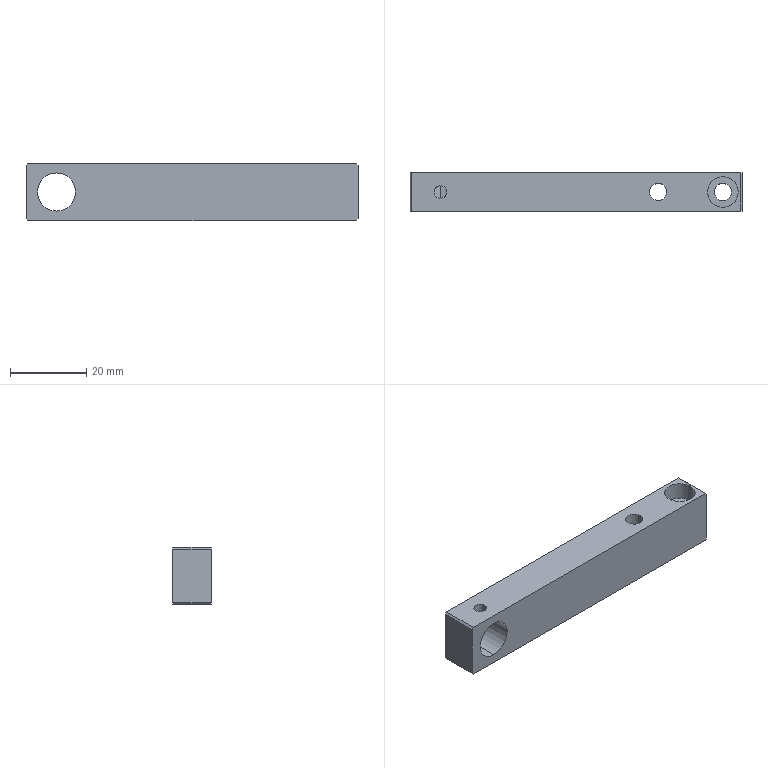Part | SolidWorks | features HoleWzd 3, Chamfer 1, Extrusion 1, ICE 1 | 1 solid | 21 faces | box 87 x 10 x 15 mm | volume 11602 mm3 | plane 11 | cylinder 10 | commonest cylinder face diameters 4.5 x4 3.3 x2 8 x2 10 x2
STEP:
#1=CARTESIAN_POINT('',(-37.15,5.,4.72));
#2=VERTEX_POINT('',#1);
#3=CARTESIAN_POINT('',(-35.5,3.35,5.));
#4=VERTEX_POINT('',#3);
#5=CARTESIAN_POINT('',(-37.15,5.,4.72));
#6=CARTESIAN_POINT('',(-37.15,4.891,4.72));
#7=CARTESIAN_POINT('',(-37.139,4.784,4.724));
#8=CARTESIAN_POINT('',(-37.097,4.57,4.738));
#9=CARTESIAN_POINT('',(-37.065,4.465,4.749));
#10=CARTESIAN_POINT('',(-36.941,4.167,4.789));
#11=CARTESIAN_POINT('',(-36.818,3.985,4.826));
#12=CARTESIAN_POINT('',(-36.591,3.758,4.88));
#13=CARTESIAN_POINT('',(-36.507,3.689,4.898));
#14=CARTESIAN_POINT('',(-36.329,3.569,4.932));
#15=CARTESIAN_POINT('',(-36.234,3.519,4.947));
#16=CARTESIAN_POINT('',(-36.035,3.435,4.972));
#17=CARTESIAN_POINT('',(-35.93,3.403,4.983));
#18=CARTESIAN_POINT('',(-35.718,3.361,4.996));
#19=CARTESIAN_POINT('',(-35.61,3.35,5.));
#20=CARTESIAN_POINT('',(-35.5,3.35,5.));
#21=B_SPLINE_CURVE_WITH_KNOTS('',3,(#5,#6,#7,#8,#9,#10,#11,#12,#13,#14,#15,#16,#17,#18,#19,#20),.UNSPECIFIED.,.F.,.F.,(4,2,2,2,2,2,2,4),(0.007792,0.008117,0.008441,0.009091,0.009415,0.00974,0.01006,0.01039),.UNSPECIFIED.);
#22=EDGE_CURVE('',#2,#4,#21,.T.);
#23=ORIENTED_EDGE('',*,*,#22,.F.);
#24=CARTESIAN_POINT('',(-37.15,5.,7.5));
#25=VERTEX_POINT('',#24);
#26=CARTESIAN_POINT('',(-37.15,5.,7.5));
#27=DIRECTION('',(0.,0.,1.));
#28=VECTOR('',#27,1000.);
#29=LINE('',#26,#28);
#30=EDGE_CURVE('',#2,#25,#29,.T.);
#31=ORIENTED_EDGE('',*,*,#30,.T.);
#32=CARTESIAN_POINT('',(-33.85,5.,7.5));
#33=VERTEX_POINT('',#32);
#34=CARTESIAN_POINT('',(-35.5,5.,7.5));
#35=DIRECTION('',(0.,0.,1.));
#36=DIRECTION('',(1.,0.,0.));
#37=AXIS2_PLACEMENT_3D('',#34,#35,#36);
#38=CIRCLE('',#37,1.65);
#39=EDGE_CURVE('',#25,#33,#38,.T.);
#40=ORIENTED_EDGE('',*,*,#39,.T.);
#41=CARTESIAN_POINT('',(-33.85,5.,4.72));
#42=VERTEX_POINT('',#41);
#43=CARTESIAN_POINT('',(-33.85,5.,7.5));
#44=DIRECTION('',(0.,0.,1.));
#45=VECTOR('',#44,1000.);
#46=LINE('',#43,#45);
#47=EDGE_CURVE('',#42,#33,#46,.T.);
#48=ORIENTED_EDGE('',*,*,#47,.F.);
#49=CARTESIAN_POINT('',(-35.5,3.35,5.));
#50=CARTESIAN_POINT('',(-35.39,3.35,5.));
#51=CARTESIAN_POINT('',(-35.282,3.361,4.996));
#52=CARTESIAN_POINT('',(-35.07,3.403,4.983));
#53=CARTESIAN_POINT('',(-34.965,3.435,4.972));
#54=CARTESIAN_POINT('',(-34.765,3.519,4.947));
#55=CARTESIAN_POINT('',(-34.671,3.569,4.932));
#56=CARTESIAN_POINT('',(-34.492,3.689,4.898));
#57=CARTESIAN_POINT('',(-34.408,3.758,4.88));
#58=CARTESIAN_POINT('',(-34.181,3.985,4.826));
#59=CARTESIAN_POINT('',(-34.059,4.168,4.789));
#60=CARTESIAN_POINT('',(-33.935,4.466,4.749));
#61=CARTESIAN_POINT('',(-33.903,4.57,4.738));
#62=CARTESIAN_POINT('',(-33.861,4.784,4.724));
#63=CARTESIAN_POINT('',(-33.85,4.891,4.72));
#64=CARTESIAN_POINT('',(-33.85,5.,4.72));
#65=B_SPLINE_CURVE_WITH_KNOTS('',3,(#49,#50,#51,#52,#53,#54,#55,#56,#57,#58,#59,#60,#61,#62,#63,#64),.UNSPECIFIED.,.F.,.F.,(4,2,2,2,2,2,2,4),(0.,0.0003248,0.0006496,0.0009744,0.001299,0.001949,0.002274,0.002598),.UNSPECIFIED.);
#66=EDGE_CURVE('',#4,#42,#65,.T.);
#67=ORIENTED_EDGE('',*,*,#66,.F.);
#68=EDGE_LOOP('',(#23,#31,#40,#48,#67));
#69=FACE_OUTER_BOUND('',#68,.T.);
#70=CARTESIAN_POINT('',(-35.5,5.,7.5));
#71=DIRECTION('',(0.,0.,1.));
#72=DIRECTION('',(1.,0.,0.));
#73=AXIS2_PLACEMENT_3D('',#70,#71,#72);
#74=CYLINDRICAL_SURFACE('',#73,1.65);
#75=ADVANCED_FACE('',(#69),#74,.F.);
#76=CARTESIAN_POINT('',(34.5,5.,2.9));
#77=VERTEX_POINT('',#76);
#78=CARTESIAN_POINT('',(42.5,5.,2.9));
#79=VERTEX_POINT('',#78);
#80=CARTESIAN_POINT('',(38.5,5.,2.9));
#81=DIRECTION('',(0.,0.,1.));
#82=DIRECTION('',(1.,0.,0.));
#83=AXIS2_PLACEMENT_3D('',#80,#81,#82);
#84=CIRCLE('',#83,4.);
#85=EDGE_CURVE('',#77,#79,#84,.T.);
#86=ORIENTED_EDGE('',*,*,#85,.F.);
#87=CARTESIAN_POINT('',(34.5,5.,7.5));
#88=VERTEX_POINT('',#87);
#89=CARTESIAN_POINT('',(34.5,5.,7.5));
#90=DIRECTION('',(0.,0.,1.));
#91=VECTOR('',#90,1000.);
#92=LINE('',#89,#91);
#93=EDGE_CURVE('',#77,#88,#92,.T.);
#94=ORIENTED_EDGE('',*,*,#93,.T.);
#95=CARTESIAN_POINT('',(42.5,5.,7.5));
#96=VERTEX_POINT('',#95);
#97=CARTESIAN_POINT('',(38.5,5.,7.5));
#98=DIRECTION('',(0.,0.,1.));
#99=DIRECTION('',(1.,0.,0.));
#100=AXIS2_PLACEMENT_3D('',#97,#98,#99);
#101=CIRCLE('',#100,4.);
#102=EDGE_CURVE('',#88,#96,#101,.T.);
#103=ORIENTED_EDGE('',*,*,#102,.T.);
#104=CARTESIAN_POINT('',(42.5,5.,7.5));
#105=DIRECTION('',(0.,0.,1.));
#106=VECTOR('',#105,1000.);
#107=LINE('',#104,#106);
#108=EDGE_CURVE('',#79,#96,#107,.T.);
#109=ORIENTED_EDGE('',*,*,#108,.F.);
#110=EDGE_LOOP('',(#86,#94,#103,#109));
#111=FACE_OUTER_BOUND('',#110,.T.);
#112=CARTESIAN_POINT('',(38.5,5.,7.5));
#113=DIRECTION('',(0.,0.,1.));
#114=DIRECTION('',(1.,0.,0.));
#115=AXIS2_PLACEMENT_3D('',#112,#113,#114);
#116=CYLINDRICAL_SURFACE('',#115,4.);
#117=ADVANCED_FACE('',(#111),#116,.F.);
#118=CARTESIAN_POINT('',(36.25,5.,-7.5));
#119=VERTEX_POINT('',#118);
#120=CARTESIAN_POINT('',(40.75,5.,-7.5));
#121=VERTEX_POINT('',#120);
#122=CARTESIAN_POINT('',(38.5,5.,-7.5));
#123=DIRECTION('',(0.,0.,1.));
#124=DIRECTION('',(1.,0.,0.));
#125=AXIS2_PLACEMENT_3D('',#122,#123,#124);
#126=CIRCLE('',#125,2.25);
#127=EDGE_CURVE('',#119,#121,#126,.T.);
#128=ORIENTED_EDGE('',*,*,#127,.F.);
#129=CARTESIAN_POINT('',(36.25,5.,2.9));
#130=VERTEX_POINT('',#129);
#131=CARTESIAN_POINT('',(36.25,5.,7.5));
#132=DIRECTION('',(0.,0.,1.));
#133=VECTOR('',#132,1000.);
#134=LINE('',#131,#133);
#135=EDGE_CURVE('',#119,#130,#134,.T.);
#136=ORIENTED_EDGE('',*,*,#135,.T.);
#137=CARTESIAN_POINT('',(40.75,5.,2.9));
#138=VERTEX_POINT('',#137);
#139=CARTESIAN_POINT('',(38.5,5.,2.9));
#140=DIRECTION('',(0.,0.,1.));
#141=DIRECTION('',(1.,0.,0.));
#142=AXIS2_PLACEMENT_3D('',#139,#140,#141);
#143=CIRCLE('',#142,2.25);
#144=EDGE_CURVE('',#130,#138,#143,.T.);
#145=ORIENTED_EDGE('',*,*,#144,.T.);
#146=CARTESIAN_POINT('',(40.75,5.,7.5));
#147=DIRECTION('',(0.,0.,1.));
#148=VECTOR('',#147,1000.);
#149=LINE('',#146,#148);
#150=EDGE_CURVE('',#121,#138,#149,.T.);
#151=ORIENTED_EDGE('',*,*,#150,.F.);
#152=EDGE_LOOP('',(#128,#136,#145,#151));
#153=FACE_OUTER_BOUND('',#152,.T.);
#154=CARTESIAN_POINT('',(38.5,5.,7.5));
#155=DIRECTION('',(0.,0.,1.));
#156=DIRECTION('',(1.,0.,0.));
#157=AXIS2_PLACEMENT_3D('',#154,#155,#156);
#158=CYLINDRICAL_SURFACE('',#157,2.25);
#159=ADVANCED_FACE('',(#153),#158,.F.);
#160=CARTESIAN_POINT('',(23.75,5.,7.5));
#161=VERTEX_POINT('',#160);
#162=CARTESIAN_POINT('',(19.25,5.,7.5));
#163=VERTEX_POINT('',#162);
#164=CARTESIAN_POINT('',(21.5,5.,7.5));
#165=DIRECTION('',(0.,0.,-1.));
#166=DIRECTION('',(-1.,0.,0.));
#167=AXIS2_PLACEMENT_3D('',#164,#165,#166);
#168=CIRCLE('',#167,2.25);
#169=EDGE_CURVE('',#161,#163,#168,.T.);
#170=ORIENTED_EDGE('',*,*,#169,.F.);
#171=CARTESIAN_POINT('',(23.75,5.,-7.5));
#172=VERTEX_POINT('',#171);
#173=CARTESIAN_POINT('',(23.75,5.,-7.5));
#174=DIRECTION('',(0.,0.,-1.));
#175=VECTOR('',#174,1000.);
#176=LINE('',#173,#175);
#177=EDGE_CURVE('',#161,#172,#176,.T.);
#178=ORIENTED_EDGE('',*,*,#177,.T.);
#179=CARTESIAN_POINT('',(19.25,5.,-7.5));
#180=VERTEX_POINT('',#179);
#181=CARTESIAN_POINT('',(21.5,5.,-7.5));
#182=DIRECTION('',(0.,0.,-1.));
#183=DIRECTION('',(-1.,0.,0.));
#184=AXIS2_PLACEMENT_3D('',#181,#182,#183);
#185=CIRCLE('',#184,2.25);
#186=EDGE_CURVE('',#172,#180,#185,.T.);
#187=ORIENTED_EDGE('',*,*,#186,.T.);
#188=CARTESIAN_POINT('',(19.25,5.,-7.5));
#189=DIRECTION('',(0.,0.,-1.));
#190=VECTOR('',#189,1000.);
#191=LINE('',#188,#190);
#192=EDGE_CURVE('',#163,#180,#191,.T.);
#193=ORIENTED_EDGE('',*,*,#192,.F.);
#194=EDGE_LOOP('',(#170,#178,#187,#193));
#195=FACE_OUTER_BOUND('',#194,.T.);
#196=CARTESIAN_POINT('',(21.5,5.,-7.5));
#197=DIRECTION('',(0.,0.,-1.));
#198=DIRECTION('',(-1.,0.,0.));
#199=AXIS2_PLACEMENT_3D('',#196,#197,#198);
#200=CYLINDRICAL_SURFACE('',#199,2.25);
#201=ADVANCED_FACE('',(#195),#200,.F.);
#202=CARTESIAN_POINT('',(-35.5,0.,-5.));
#203=VERTEX_POINT('',#202);
#204=CARTESIAN_POINT('',(-35.5,0.,5.));
#205=VERTEX_POINT('',#204);
#206=CARTESIAN_POINT('',(-35.5,0.,0.));
#207=DIRECTION('',(0.,1.,0.));
#208=DIRECTION('',(0.,0.,1.));
#209=AXIS2_PLACEMENT_3D('',#206,#207,#208);
#210=CIRCLE('',#209,5.);
#211=EDGE_CURVE('',#203,#205,#210,.T.);
#212=ORIENTED_EDGE('',*,*,#211,.F.);
#213=CARTESIAN_POINT('',(-35.5,10.,-5.));
#214=VERTEX_POINT('',#213);
#215=CARTESIAN_POINT('',(-35.5,0.,-5.));
#216=DIRECTION('',(0.,1.,0.));
#217=VECTOR('',#216,1000.);
#218=LINE('',#215,#217);
#219=EDGE_CURVE('',#203,#214,#218,.T.);
#220=ORIENTED_EDGE('',*,*,#219,.T.);
#221=CARTESIAN_POINT('',(-35.5,10.,5.));
#222=VERTEX_POINT('',#221);
#223=CARTESIAN_POINT('',(-35.5,10.,0.));
#224=DIRECTION('',(0.,1.,0.));
#225=DIRECTION('',(0.,0.,1.));
#226=AXIS2_PLACEMENT_3D('',#223,#224,#225);
#227=CIRCLE('',#226,5.);
#228=EDGE_CURVE('',#214,#222,#227,.T.);
#229=ORIENTED_EDGE('',*,*,#228,.T.);
#230=CARTESIAN_POINT('',(-35.5,6.65,5.));
#231=VERTEX_POINT('',#230);
#232=CARTESIAN_POINT('',(-35.5,0.,5.));
#233=DIRECTION('',(0.,1.,0.));
#234=VECTOR('',#233,1000.);
#235=LINE('',#232,#234);
#236=EDGE_CURVE('',#231,#222,#235,.T.);
#237=ORIENTED_EDGE('',*,*,#236,.F.);
#238=CARTESIAN_POINT('',(-35.5,6.65,5.));
#239=CARTESIAN_POINT('',(-35.716,6.65,5.));
#240=CARTESIAN_POINT('',(-35.935,6.606,4.985));
#241=CARTESIAN_POINT('',(-36.233,6.482,4.947));
#242=CARTESIAN_POINT('',(-36.33,6.43,4.931));
#243=CARTESIAN_POINT('',(-36.508,6.311,4.898));
#244=CARTESIAN_POINT('',(-36.591,6.243,4.88));
#245=CARTESIAN_POINT('',(-36.819,6.014,4.825));
#246=CARTESIAN_POINT('',(-36.94,5.834,4.789));
#247=CARTESIAN_POINT('',(-37.065,5.534,4.749));
#248=CARTESIAN_POINT('',(-37.097,5.43,4.738));
#249=CARTESIAN_POINT('',(-37.139,5.219,4.724));
#250=CARTESIAN_POINT('',(-37.15,5.109,4.72));
#251=CARTESIAN_POINT('',(-37.15,5.,4.72));
#252=B_SPLINE_CURVE_WITH_KNOTS('',3,(#238,#239,#240,#241,#242,#243,#244,#245,#246,#247,#248,#249,#250,#251),.UNSPECIFIED.,.F.,.F.,(4,2,2,2,2,2,4),(0.005195,0.005845,0.006169,0.006494,0.007143,0.007468,0.007792),.UNSPECIFIED.);
#253=EDGE_CURVE('',#231,#2,#252,.T.);
#254=ORIENTED_EDGE('',*,*,#253,.T.);
#255=ORIENTED_EDGE('',*,*,#22,.T.);
#256=CARTESIAN_POINT('',(-35.5,0.,5.));
#257=DIRECTION('',(0.,1.,0.));
#258=VECTOR('',#257,1000.);
#259=LINE('',#256,#258);
#260=EDGE_CURVE('',#205,#4,#259,.T.);
#261=ORIENTED_EDGE('',*,*,#260,.F.);
#262=EDGE_LOOP('',(#212,#220,#229,#237,#254,#255,#261));
#263=FACE_OUTER_BOUND('',#262,.T.);
#264=CARTESIAN_POINT('',(-35.5,0.,0.));
#265=DIRECTION('',(0.,1.,0.));
#266=DIRECTION('',(0.,0.,1.));
#267=AXIS2_PLACEMENT_3D('',#264,#265,#266);
#268=CYLINDRICAL_SURFACE('',#267,5.);
#269=ADVANCED_FACE('',(#263),#268,.F.);
#270=CARTESIAN_POINT('',(-43.5,10.,-7.));
#271=VERTEX_POINT('',#270);
#272=CARTESIAN_POINT('',(-43.5,10.,7.));
#273=VERTEX_POINT('',#272);
#274=CARTESIAN_POINT('',(-43.5,10.,-7.5));
#275=DIRECTION('',(0.,0.,1.));
#276=VECTOR('',#275,1000.);
#277=LINE('',#274,#276);
#278=EDGE_CURVE('',#271,#273,#277,.T.);
#279=ORIENTED_EDGE('',*,*,#278,.F.);
#280=CARTESIAN_POINT('',(-43.5,0.,-7.));
#281=VERTEX_POINT('',#280);
#282=CARTESIAN_POINT('',(-43.5,0.,-7.));
#283=DIRECTION('',(0.,-1.,0.));
#284=VECTOR('',#283,1000.);
#285=LINE('',#282,#284);
#286=EDGE_CURVE('',#271,#281,#285,.T.);
#287=ORIENTED_EDGE('',*,*,#286,.T.);
#288=CARTESIAN_POINT('',(-43.5,0.,7.));
#289=VERTEX_POINT('',#288);
#290=CARTESIAN_POINT('',(-43.5,0.,-7.5));
#291=DIRECTION('',(0.,0.,1.));
#292=VECTOR('',#291,1000.);
#293=LINE('',#290,#292);
#294=EDGE_CURVE('',#281,#289,#293,.T.);
#295=ORIENTED_EDGE('',*,*,#294,.T.);
#296=CARTESIAN_POINT('',(-43.5,10.,7.));
#297=DIRECTION('',(0.,1.,0.));
#298=VECTOR('',#297,1000.);
#299=LINE('',#296,#298);
#300=EDGE_CURVE('',#289,#273,#299,.T.);
#301=ORIENTED_EDGE('',*,*,#300,.T.);
#302=EDGE_LOOP('',(#279,#287,#295,#301));
#303=FACE_OUTER_BOUND('',#302,.T.);
#304=CARTESIAN_POINT('',(-43.5,10.,-7.5));
#305=DIRECTION('',(1.,0.,0.));
#306=DIRECTION('',(0.,0.,-1.));
#307=AXIS2_PLACEMENT_3D('',#304,#305,#306);
#308=PLANE('',#307);
#309=ADVANCED_FACE('',(#303),#308,.F.);
#310=CARTESIAN_POINT('',(-35.5,5.,7.5));
#311=DIRECTION('',(0.,0.,1.));
#312=DIRECTION('',(1.,0.,0.));
#313=AXIS2_PLACEMENT_3D('',#310,#311,#312);
#314=CIRCLE('',#313,1.65);
#315=EDGE_CURVE('',#33,#25,#314,.T.);
#316=ORIENTED_EDGE('',*,*,#315,.F.);
#317=ORIENTED_EDGE('',*,*,#39,.F.);
#318=EDGE_LOOP('',(#316,#317));
#319=FACE_BOUND('',#318,.T.);
#320=CARTESIAN_POINT('',(38.5,5.,7.5));
#321=DIRECTION('',(0.,0.,1.));
#322=DIRECTION('',(1.,0.,0.));
#323=AXIS2_PLACEMENT_3D('',#320,#321,#322);
#324=CIRCLE('',#323,4.);
#325=EDGE_CURVE('',#96,#88,#324,.T.);
#326=ORIENTED_EDGE('',*,*,#325,.F.);
#327=ORIENTED_EDGE('',*,*,#102,.F.);
#328=EDGE_LOOP('',(#326,#327));
#329=FACE_BOUND('',#328,.T.);
#330=CARTESIAN_POINT('',(21.5,5.,7.5));
#331=DIRECTION('',(0.,0.,-1.));
#332=DIRECTION('',(-1.,0.,0.));
#333=AXIS2_PLACEMENT_3D('',#330,#331,#332);
#334=CIRCLE('',#333,2.25);
#335=EDGE_CURVE('',#163,#161,#334,.T.);
#336=ORIENTED_EDGE('',*,*,#335,.T.);
#337=ORIENTED_EDGE('',*,*,#169,.T.);
#338=EDGE_LOOP('',(#336,#337));
#339=FACE_BOUND('',#338,.T.);
#340=CARTESIAN_POINT('',(-43.,0.,7.5));
#341=VERTEX_POINT('',#340);
#342=CARTESIAN_POINT('',(43.,0.,7.5));
#343=VERTEX_POINT('',#342);
#344=CARTESIAN_POINT('',(-43.5,0.,7.5));
#345=DIRECTION('',(1.,0.,0.));
#346=VECTOR('',#345,1000.);
#347=LINE('',#344,#346);
#348=EDGE_CURVE('',#341,#343,#347,.T.);
#349=ORIENTED_EDGE('',*,*,#348,.T.);
#350=CARTESIAN_POINT('',(43.,10.,7.5));
#351=VERTEX_POINT('',#350);
#352=CARTESIAN_POINT('',(43.,10.,7.5));
#353=DIRECTION('',(0.,1.,0.));
#354=VECTOR('',#353,1000.);
#355=LINE('',#352,#354);
#356=EDGE_CURVE('',#343,#351,#355,.T.);
#357=ORIENTED_EDGE('',*,*,#356,.T.);
#358=CARTESIAN_POINT('',(-43.,10.,7.5));
#359=VERTEX_POINT('',#358);
#360=CARTESIAN_POINT('',(-43.5,10.,7.5));
#361=DIRECTION('',(1.,0.,0.));
#362=VECTOR('',#361,1000.);
#363=LINE('',#360,#362);
#364=EDGE_CURVE('',#359,#351,#363,.T.);
#365=ORIENTED_EDGE('',*,*,#364,.F.);
#366=CARTESIAN_POINT('',(-43.,10.,7.5));
#367=DIRECTION('',(0.,-1.,0.));
#368=VECTOR('',#367,1000.);
#369=LINE('',#366,#368);
#370=EDGE_CURVE('',#359,#341,#369,.T.);
#371=ORIENTED_EDGE('',*,*,#370,.T.);
#372=EDGE_LOOP('',(#349,#357,#365,#371));
#373=FACE_OUTER_BOUND('',#372,.T.);
#374=CARTESIAN_POINT('',(-43.5,10.,7.5));
#375=DIRECTION('',(0.,0.,-1.));
#376=DIRECTION('',(-1.,0.,0.));
#377=AXIS2_PLACEMENT_3D('',#374,#375,#376);
#378=PLANE('',#377);
#379=ADVANCED_FACE('',(#319,#329,#339,#373),#378,.F.);
#380=CARTESIAN_POINT('',(43.5,0.,-7.));
#381=VERTEX_POINT('',#380);
#382=CARTESIAN_POINT('',(43.5,0.,7.));
#383=VERTEX_POINT('',#382);
#384=CARTESIAN_POINT('',(43.5,0.,-7.5));
#385=DIRECTION('',(0.,0.,1.));
#386=VECTOR('',#385,1000.);
#387=LINE('',#384,#386);
#388=EDGE_CURVE('',#381,#383,#387,.T.);
#389=ORIENTED_EDGE('',*,*,#388,.F.);
#390=CARTESIAN_POINT('',(43.5,10.,-7.));
#391=VERTEX_POINT('',#390);
#392=CARTESIAN_POINT('',(43.5,10.,-7.));
#393=DIRECTION('',(0.,1.,0.));
#394=VECTOR('',#393,1000.);
#395=LINE('',#392,#394);
#396=EDGE_CURVE('',#381,#391,#395,.T.);
#397=ORIENTED_EDGE('',*,*,#396,.T.);
#398=CARTESIAN_POINT('',(43.5,10.,7.));
#399=VERTEX_POINT('',#398);
#400=CARTESIAN_POINT('',(43.5,10.,-7.5));
#401=DIRECTION('',(0.,0.,1.));
#402=VECTOR('',#401,1000.);
#403=LINE('',#400,#402);
#404=EDGE_CURVE('',#391,#399,#403,.T.);
#405=ORIENTED_EDGE('',*,*,#404,.T.);
#406=CARTESIAN_POINT('',(43.5,0.,7.));
#407=DIRECTION('',(0.,-1.,0.));
#408=VECTOR('',#407,1000.);
#409=LINE('',#406,#408);
#410=EDGE_CURVE('',#399,#383,#409,.T.);
#411=ORIENTED_EDGE('',*,*,#410,.T.);
#412=EDGE_LOOP('',(#389,#397,#405,#411));
#413=FACE_OUTER_BOUND('',#412,.T.);
#414=CARTESIAN_POINT('',(43.5,10.,-7.5));
#415=DIRECTION('',(1.,0.,0.));
#416=DIRECTION('',(0.,0.,-1.));
#417=AXIS2_PLACEMENT_3D('',#414,#415,#416);
#418=PLANE('',#417);
#419=ADVANCED_FACE('',(#413),#418,.T.);
#420=CARTESIAN_POINT('',(38.5,5.,-7.5));
#421=DIRECTION('',(0.,0.,1.));
#422=DIRECTION('',(1.,0.,0.));
#423=AXIS2_PLACEMENT_3D('',#420,#421,#422);
#424=CIRCLE('',#423,2.25);
#425=EDGE_CURVE('',#121,#119,#424,.T.);
#426=ORIENTED_EDGE('',*,*,#425,.T.);
#427=ORIENTED_EDGE('',*,*,#127,.T.);
#428=EDGE_LOOP('',(#426,#427));
#429=FACE_BOUND('',#428,.T.);
#430=CARTESIAN_POINT('',(21.5,5.,-7.5));
#431=DIRECTION('',(0.,0.,-1.));
#432=DIRECTION('',(-1.,0.,0.));
#433=AXIS2_PLACEMENT_3D('',#430,#431,#432);
#434=CIRCLE('',#433,2.25);
#435=EDGE_CURVE('',#180,#172,#434,.T.);
#436=ORIENTED_EDGE('',*,*,#435,.F.);
#437=ORIENTED_EDGE('',*,*,#186,.F.);
#438=EDGE_LOOP('',(#436,#437));
#439=FACE_BOUND('',#438,.T.);
#440=CARTESIAN_POINT('',(-43.,10.,-7.5));
#441=VERTEX_POINT('',#440);
#442=CARTESIAN_POINT('',(43.,10.,-7.5));
#443=VERTEX_POINT('',#442);
#444=CARTESIAN_POINT('',(-43.5,10.,-7.5));
#445=DIRECTION('',(1.,0.,0.));
#446=VECTOR('',#445,1000.);
#447=LINE('',#444,#446);
#448=EDGE_CURVE('',#441,#443,#447,.T.);
#449=ORIENTED_EDGE('',*,*,#448,.T.);
#450=CARTESIAN_POINT('',(43.,0.,-7.5));
#451=VERTEX_POINT('',#450);
#452=CARTESIAN_POINT('',(43.,10.,-7.5));
#453=DIRECTION('',(0.,-1.,0.));
#454=VECTOR('',#453,1000.);
#455=LINE('',#452,#454);
#456=EDGE_CURVE('',#443,#451,#455,.T.);
#457=ORIENTED_EDGE('',*,*,#456,.T.);
#458=CARTESIAN_POINT('',(-43.,0.,-7.5));
#459=VERTEX_POINT('',#458);
#460=CARTESIAN_POINT('',(-43.5,0.,-7.5));
#461=DIRECTION('',(1.,0.,0.));
#462=VECTOR('',#461,1000.);
#463=LINE('',#460,#462);
#464=EDGE_CURVE('',#459,#451,#463,.T.);
#465=ORIENTED_EDGE('',*,*,#464,.F.);
#466=CARTESIAN_POINT('',(-43.,10.,-7.5));
#467=DIRECTION('',(0.,1.,0.));
#468=VECTOR('',#467,1000.);
#469=LINE('',#466,#468);
#470=EDGE_CURVE('',#459,#441,#469,.T.);
#471=ORIENTED_EDGE('',*,*,#470,.T.);
#472=EDGE_LOOP('',(#449,#457,#465,#471));
#473=FACE_OUTER_BOUND('',#472,.T.);
#474=CARTESIAN_POINT('',(-43.5,10.,-7.5));
#475=DIRECTION('',(0.,0.,-1.));
#476=DIRECTION('',(-1.,0.,0.));
#477=AXIS2_PLACEMENT_3D('',#474,#475,#476);
#478=PLANE('',#477);
#479=ADVANCED_FACE('',(#429,#439,#473),#478,.T.);
#480=CARTESIAN_POINT('',(-35.5,10.,0.));
#481=DIRECTION('',(0.,1.,0.));
#482=DIRECTION('',(0.,0.,1.));
#483=AXIS2_PLACEMENT_3D('',#480,#481,#482);
#484=CIRCLE('',#483,5.);
#485=EDGE_CURVE('',#222,#214,#484,.T.);
#486=ORIENTED_EDGE('',*,*,#485,.F.);
#487=ORIENTED_EDGE('',*,*,#228,.F.);
#488=EDGE_LOOP('',(#486,#487));
#489=FACE_BOUND('',#488,.T.);
#490=ORIENTED_EDGE('',*,*,#404,.F.);
#491=CARTESIAN_POINT('',(25.25,10.,-25.25));
#492=DIRECTION('',(-0.7071,0.,-0.7071));
#493=VECTOR('',#492,1000.);
#494=LINE('',#491,#493);
#495=EDGE_CURVE('',#391,#443,#494,.T.);
#496=ORIENTED_EDGE('',*,*,#495,.T.);
#497=ORIENTED_EDGE('',*,*,#448,.F.);
#498=CARTESIAN_POINT('',(-25.25,10.,-25.25));
#499=DIRECTION('',(-0.7071,0.,0.7071));
#500=VECTOR('',#499,1000.);
#501=LINE('',#498,#500);
#502=EDGE_CURVE('',#441,#271,#501,.T.);
#503=ORIENTED_EDGE('',*,*,#502,.T.);
#504=ORIENTED_EDGE('',*,*,#278,.T.);
#505=CARTESIAN_POINT('',(-25.25,10.,25.25));
#506=DIRECTION('',(0.7071,0.,0.7071));
#507=VECTOR('',#506,1000.);
#508=LINE('',#505,#507);
#509=EDGE_CURVE('',#273,#359,#508,.T.);
#510=ORIENTED_EDGE('',*,*,#509,.T.);
#511=ORIENTED_EDGE('',*,*,#364,.T.);
#512=CARTESIAN_POINT('',(25.25,10.,25.25));
#513=DIRECTION('',(0.7071,0.,-0.7071));
#514=VECTOR('',#513,1000.);
#515=LINE('',#512,#514);
#516=EDGE_CURVE('',#351,#399,#515,.T.);
#517=ORIENTED_EDGE('',*,*,#516,.T.);
#518=EDGE_LOOP('',(#490,#496,#497,#503,#504,#510,#511,#517));
#519=FACE_OUTER_BOUND('',#518,.T.);
#520=CARTESIAN_POINT('',(0.,10.,0.));
#521=DIRECTION('',(0.,1.,0.));
#522=DIRECTION('',(0.,0.,1.));
#523=AXIS2_PLACEMENT_3D('',#520,#521,#522);
#524=PLANE('',#523);
#525=ADVANCED_FACE('',(#489,#519),#524,.T.);
#526=CARTESIAN_POINT('',(-35.5,0.,0.));
#527=DIRECTION('',(0.,1.,0.));
#528=DIRECTION('',(0.,0.,1.));
#529=AXIS2_PLACEMENT_3D('',#526,#527,#528);
#530=CIRCLE('',#529,5.);
#531=EDGE_CURVE('',#205,#203,#530,.T.);
#532=ORIENTED_EDGE('',*,*,#531,.T.);
#533=ORIENTED_EDGE('',*,*,#211,.T.);
#534=EDGE_LOOP('',(#532,#533));
#535=FACE_BOUND('',#534,.T.);
#536=ORIENTED_EDGE('',*,*,#464,.T.);
#537=CARTESIAN_POINT('',(43.,0.,-7.5));
#538=DIRECTION('',(0.7071,0.,0.7071));
#539=VECTOR('',#538,1000.);
#540=LINE('',#537,#539);
#541=EDGE_CURVE('',#451,#381,#540,.T.);
#542=ORIENTED_EDGE('',*,*,#541,.T.);
#543=ORIENTED_EDGE('',*,*,#388,.T.);
#544=CARTESIAN_POINT('',(43.5,0.,7.));
#545=DIRECTION('',(-0.7071,0.,0.7071));
#546=VECTOR('',#545,1000.);
#547=LINE('',#544,#546);
#548=EDGE_CURVE('',#383,#343,#547,.T.);
#549=ORIENTED_EDGE('',*,*,#548,.T.);
#550=ORIENTED_EDGE('',*,*,#348,.F.);
#551=CARTESIAN_POINT('',(-43.,0.,7.5));
#552=DIRECTION('',(-0.7071,0.,-0.7071));
#553=VECTOR('',#552,1000.);
#554=LINE('',#551,#553);
#555=EDGE_CURVE('',#341,#289,#554,.T.);
#556=ORIENTED_EDGE('',*,*,#555,.T.);
#557=ORIENTED_EDGE('',*,*,#294,.F.);
#558=CARTESIAN_POINT('',(-43.5,0.,-7.));
#559=DIRECTION('',(0.7071,0.,-0.7071));
#560=VECTOR('',#559,1000.);
#561=LINE('',#558,#560);
#562=EDGE_CURVE('',#281,#459,#561,.T.);
#563=ORIENTED_EDGE('',*,*,#562,.T.);
#564=EDGE_LOOP('',(#536,#542,#543,#549,#550,#556,#557,#563));
#565=FACE_OUTER_BOUND('',#564,.T.);
#566=CARTESIAN_POINT('',(0.,0.,0.));
#567=DIRECTION('',(0.,1.,0.));
#568=DIRECTION('',(0.,0.,1.));
#569=AXIS2_PLACEMENT_3D('',#566,#567,#568);
#570=PLANE('',#569);
#571=ADVANCED_FACE('',(#535,#565),#570,.F.);
#572=ORIENTED_EDGE('',*,*,#219,.F.);
#573=ORIENTED_EDGE('',*,*,#531,.F.);
#574=ORIENTED_EDGE('',*,*,#260,.T.);
#575=ORIENTED_EDGE('',*,*,#66,.T.);
#576=CARTESIAN_POINT('',(-33.85,5.,4.72));
#577=CARTESIAN_POINT('',(-33.85,5.108,4.72));
#578=CARTESIAN_POINT('',(-33.861,5.219,4.724));
#579=CARTESIAN_POINT('',(-33.904,5.431,4.738));
#580=CARTESIAN_POINT('',(-33.935,5.534,4.749));
#581=CARTESIAN_POINT('',(-34.06,5.835,4.789));
#582=CARTESIAN_POINT('',(-34.182,6.016,4.826));
#583=CARTESIAN_POINT('',(-34.41,6.243,4.88));
#584=CARTESIAN_POINT('',(-34.492,6.311,4.898));
#585=CARTESIAN_POINT('',(-34.671,6.43,4.932));
#586=CARTESIAN_POINT('',(-34.767,6.482,4.947));
#587=CARTESIAN_POINT('',(-35.065,6.606,4.985));
#588=CARTESIAN_POINT('',(-35.284,6.65,5.));
#589=CARTESIAN_POINT('',(-35.5,6.65,5.));
#590=B_SPLINE_CURVE_WITH_KNOTS('',3,(#576,#577,#578,#579,#580,#581,#582,#583,#584,#585,#586,#587,#588,#589),.UNSPECIFIED.,.F.,.F.,(4,2,2,2,2,2,4),(0.002598,0.002923,0.003248,0.003897,0.004222,0.004546,0.005195),.UNSPECIFIED.);
#591=EDGE_CURVE('',#42,#231,#590,.T.);
#592=ORIENTED_EDGE('',*,*,#591,.T.);
#593=ORIENTED_EDGE('',*,*,#236,.T.);
#594=ORIENTED_EDGE('',*,*,#485,.T.);
#595=EDGE_LOOP('',(#572,#573,#574,#575,#592,#593,#594));
#596=FACE_OUTER_BOUND('',#595,.T.);
#597=CARTESIAN_POINT('',(-35.5,0.,0.));
#598=DIRECTION('',(0.,1.,0.));
#599=DIRECTION('',(0.,0.,1.));
#600=AXIS2_PLACEMENT_3D('',#597,#598,#599);
#601=CYLINDRICAL_SURFACE('',#600,5.);
#602=ADVANCED_FACE('',(#596),#601,.F.);
#603=ORIENTED_EDGE('',*,*,#177,.F.);
#604=ORIENTED_EDGE('',*,*,#335,.F.);
#605=ORIENTED_EDGE('',*,*,#192,.T.);
#606=ORIENTED_EDGE('',*,*,#435,.T.);
#607=EDGE_LOOP('',(#603,#604,#605,#606));
#608=FACE_OUTER_BOUND('',#607,.T.);
#609=CARTESIAN_POINT('',(21.5,5.,-7.5));
#610=DIRECTION('',(0.,0.,-1.));
#611=DIRECTION('',(-1.,0.,0.));
#612=AXIS2_PLACEMENT_3D('',#609,#610,#611);
#613=CYLINDRICAL_SURFACE('',#612,2.25);
#614=ADVANCED_FACE('',(#608),#613,.F.);
#615=ORIENTED_EDGE('',*,*,#135,.F.);
#616=ORIENTED_EDGE('',*,*,#425,.F.);
#617=ORIENTED_EDGE('',*,*,#150,.T.);
#618=CARTESIAN_POINT('',(38.5,5.,2.9));
#619=DIRECTION('',(0.,0.,1.));
#620=DIRECTION('',(1.,0.,0.));
#621=AXIS2_PLACEMENT_3D('',#618,#619,#620);
#622=CIRCLE('',#621,2.25);
#623=EDGE_CURVE('',#138,#130,#622,.T.);
#624=ORIENTED_EDGE('',*,*,#623,.T.);
#625=EDGE_LOOP('',(#615,#616,#617,#624));
#626=FACE_OUTER_BOUND('',#625,.T.);
#627=CARTESIAN_POINT('',(38.5,5.,7.5));
#628=DIRECTION('',(0.,0.,1.));
#629=DIRECTION('',(1.,0.,0.));
#630=AXIS2_PLACEMENT_3D('',#627,#628,#629);
#631=CYLINDRICAL_SURFACE('',#630,2.25);
#632=ADVANCED_FACE('',(#626),#631,.F.);
#633=ORIENTED_EDGE('',*,*,#623,.F.);
#634=ORIENTED_EDGE('',*,*,#144,.F.);
#635=EDGE_LOOP('',(#633,#634));
#636=FACE_BOUND('',#635,.T.);
#637=CARTESIAN_POINT('',(38.5,5.,2.9));
#638=DIRECTION('',(0.,0.,1.));
#639=DIRECTION('',(1.,0.,0.));
#640=AXIS2_PLACEMENT_3D('',#637,#638,#639);
#641=CIRCLE('',#640,4.);
#642=EDGE_CURVE('',#79,#77,#641,.T.);
#643=ORIENTED_EDGE('',*,*,#642,.T.);
#644=ORIENTED_EDGE('',*,*,#85,.T.);
#645=EDGE_LOOP('',(#643,#644));
#646=FACE_OUTER_BOUND('',#645,.T.);
#647=CARTESIAN_POINT('',(40.75,5.,2.9));
#648=DIRECTION('',(0.,0.,-1.));
#649=DIRECTION('',(-1.,0.,0.));
#650=AXIS2_PLACEMENT_3D('',#647,#648,#649);
#651=PLANE('',#650);
#652=ADVANCED_FACE('',(#636,#646),#651,.F.);
#653=ORIENTED_EDGE('',*,*,#93,.F.);
#654=ORIENTED_EDGE('',*,*,#642,.F.);
#655=ORIENTED_EDGE('',*,*,#108,.T.);
#656=ORIENTED_EDGE('',*,*,#325,.T.);
#657=EDGE_LOOP('',(#653,#654,#655,#656));
#658=FACE_OUTER_BOUND('',#657,.T.);
#659=CARTESIAN_POINT('',(38.5,5.,7.5));
#660=DIRECTION('',(0.,0.,1.));
#661=DIRECTION('',(1.,0.,0.));
#662=AXIS2_PLACEMENT_3D('',#659,#660,#661);
#663=CYLINDRICAL_SURFACE('',#662,4.);
#664=ADVANCED_FACE('',(#658),#663,.F.);
#665=ORIENTED_EDGE('',*,*,#495,.F.);
#666=ORIENTED_EDGE('',*,*,#396,.F.);
#667=ORIENTED_EDGE('',*,*,#541,.F.);
#668=ORIENTED_EDGE('',*,*,#456,.F.);
#669=EDGE_LOOP('',(#665,#666,#667,#668));
#670=FACE_OUTER_BOUND('',#669,.T.);
#671=CARTESIAN_POINT('',(43.,10.,-7.5));
#672=DIRECTION('',(-0.7071,0.,0.7071));
#673=DIRECTION('',(0.,-1.,0.));
#674=AXIS2_PLACEMENT_3D('',#671,#672,#673);
#675=PLANE('',#674);
#676=ADVANCED_FACE('',(#670),#675,.F.);
#677=ORIENTED_EDGE('',*,*,#516,.F.);
#678=ORIENTED_EDGE('',*,*,#356,.F.);
#679=ORIENTED_EDGE('',*,*,#548,.F.);
#680=ORIENTED_EDGE('',*,*,#410,.F.);
#681=EDGE_LOOP('',(#677,#678,#679,#680));
#682=FACE_OUTER_BOUND('',#681,.T.);
#683=CARTESIAN_POINT('',(43.5,10.,7.));
#684=DIRECTION('',(0.7071,0.,0.7071));
#685=DIRECTION('',(0.,1.,0.));
#686=AXIS2_PLACEMENT_3D('',#683,#684,#685);
#687=PLANE('',#686);
#688=ADVANCED_FACE('',(#682),#687,.T.);
#689=ORIENTED_EDGE('',*,*,#502,.F.);
#690=ORIENTED_EDGE('',*,*,#470,.F.);
#691=ORIENTED_EDGE('',*,*,#562,.F.);
#692=ORIENTED_EDGE('',*,*,#286,.F.);
#693=EDGE_LOOP('',(#689,#690,#691,#692));
#694=FACE_OUTER_BOUND('',#693,.T.);
#695=CARTESIAN_POINT('',(-43.5,10.,-7.));
#696=DIRECTION('',(-0.7071,0.,-0.7071));
#697=DIRECTION('',(0.,1.,0.));
#698=AXIS2_PLACEMENT_3D('',#695,#696,#697);
#699=PLANE('',#698);
#700=ADVANCED_FACE('',(#694),#699,.T.);
#701=ORIENTED_EDGE('',*,*,#509,.F.);
#702=ORIENTED_EDGE('',*,*,#300,.F.);
#703=ORIENTED_EDGE('',*,*,#555,.F.);
#704=ORIENTED_EDGE('',*,*,#370,.F.);
#705=EDGE_LOOP('',(#701,#702,#703,#704));
#706=FACE_OUTER_BOUND('',#705,.T.);
#707=CARTESIAN_POINT('',(-43.,10.,7.5));
#708=DIRECTION('',(0.7071,0.,-0.7071));
#709=DIRECTION('',(0.,-1.,0.));
#710=AXIS2_PLACEMENT_3D('',#707,#708,#709);
#711=PLANE('',#710);
#712=ADVANCED_FACE('',(#706),#711,.F.);
#713=ORIENTED_EDGE('',*,*,#30,.F.);
#714=ORIENTED_EDGE('',*,*,#253,.F.);
#715=ORIENTED_EDGE('',*,*,#591,.F.);
#716=ORIENTED_EDGE('',*,*,#47,.T.);
#717=ORIENTED_EDGE('',*,*,#315,.T.);
#718=EDGE_LOOP('',(#713,#714,#715,#716,#717));
#719=FACE_OUTER_BOUND('',#718,.T.);
#720=CARTESIAN_POINT('',(-35.5,5.,7.5));
#721=DIRECTION('',(0.,0.,1.));
#722=DIRECTION('',(1.,0.,0.));
#723=AXIS2_PLACEMENT_3D('',#720,#721,#722);
#724=CYLINDRICAL_SURFACE('',#723,1.65);
#725=ADVANCED_FACE('',(#719),#724,.F.);
#726=CLOSED_SHELL('',(#75,#117,#159,#201,#269,#309,#379,#419,#479,#525,#571,#602,#614,#632,#652,#664,#676,#688,#700,#712,#725));
#727=MANIFOLD_SOLID_BREP('',#726);
#728=CARTESIAN_POINT('',(0.,0.,0.));
#729=DIRECTION('',(0.,0.,1.));
#730=DIRECTION('',(1.,0.,0.));
#731=AXIS2_PLACEMENT_3D('',#728,#729,#730);
#732=(LENGTH_UNIT()NAMED_UNIT(*)SI_UNIT(.MILLI.,.METRE.));
#733=UNCERTAINTY_MEASURE_WITH_UNIT(LENGTH_MEASURE(0.00001),#732,'','');
#734=(NAMED_UNIT(*)PLANE_ANGLE_UNIT()SI_UNIT($,.RADIAN.));
#735=(NAMED_UNIT(*)SI_UNIT($,.STERADIAN.)SOLID_ANGLE_UNIT());
#736=(GEOMETRIC_REPRESENTATION_CONTEXT(3)GLOBAL_UNCERTAINTY_ASSIGNED_CONTEXT((#733))GLOBAL_UNIT_ASSIGNED_CONTEXT((#732,#734,#735))REPRESENTATION_CONTEXT('',''));
#737=ADVANCED_BREP_SHAPE_REPRESENTATION('',(#727,#731),#736);